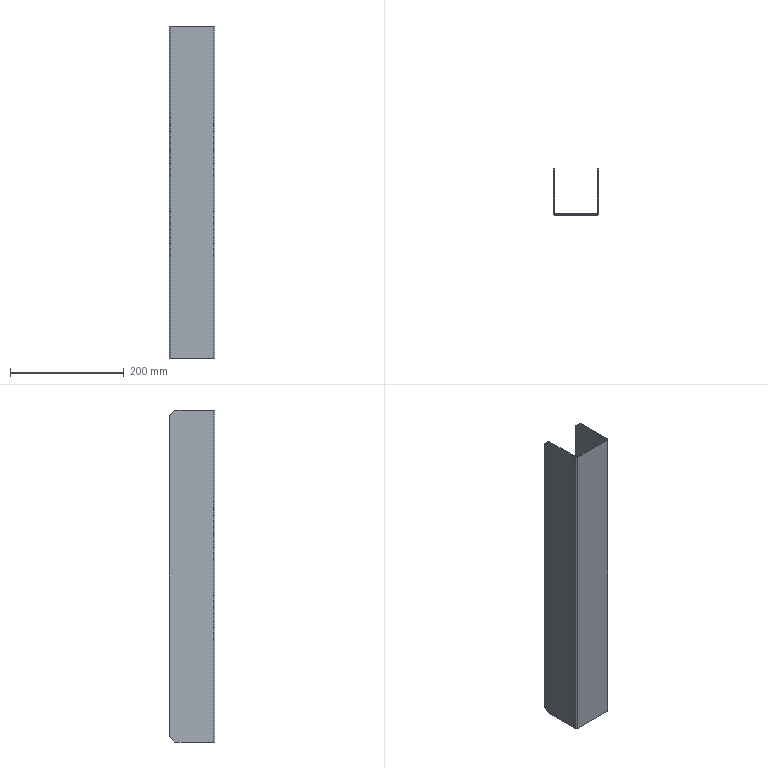Part | STEP file | SX-004-11 | 1 solid | 26 faces | box 80 x 80 x 583 mm | volume 273575 mm3 | plane 22 | cylinder 4 | commonest cylinder face diameters 0.4 x2 4.4 x2